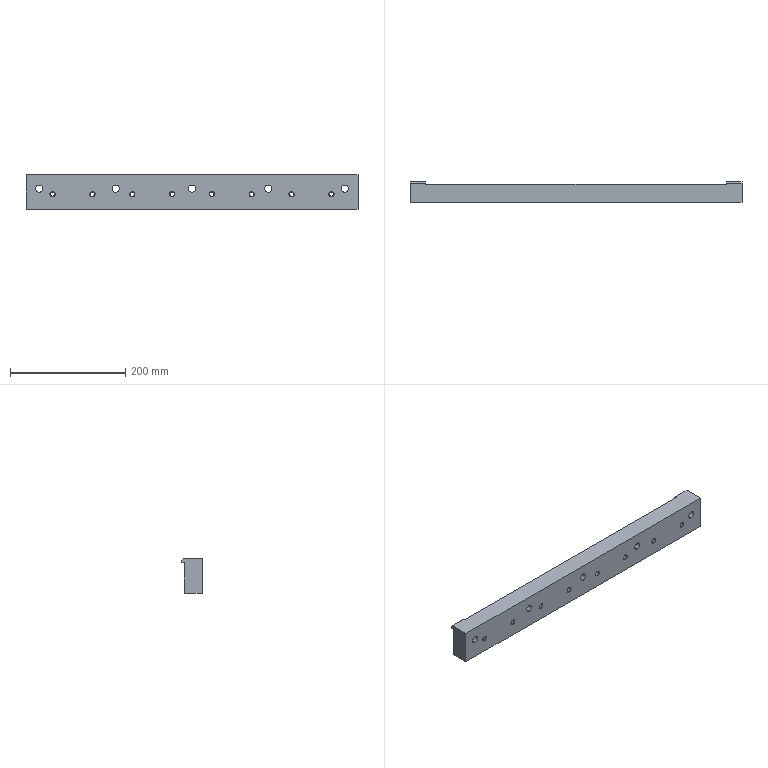Part | SolidWorks | features BaseBody 1 | 1 solid | 87 faces | box 576.923 x 35.769 x 60 mm | volume 1030017 mm3 | cylinder 36 | cone 32 | plane 19 | commonest cylinder face diameters 7.482 x16 12.692 x10 23.077 x10